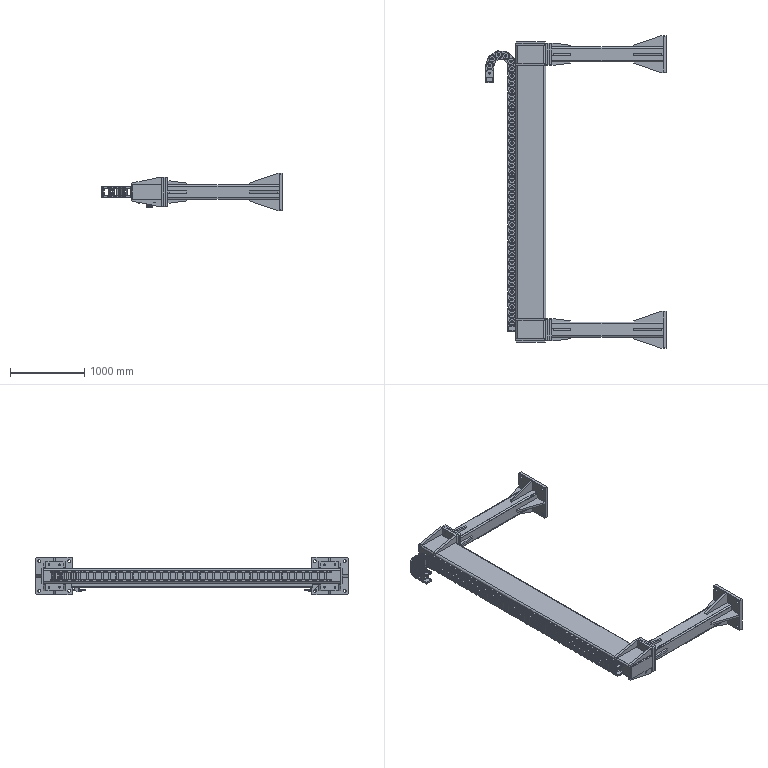Part | SolidWorks | features ReferencePattern 3, LocalLPattern 2 | 99 solids | 21928 faces | volume 164128062 mm3 | plane 12836 | cylinder 8702 | cone 390 | commonest cylinder face diameters 97 x1230 4 x520 1 x496 47.5 x488 81.7 x480 85.7 x480